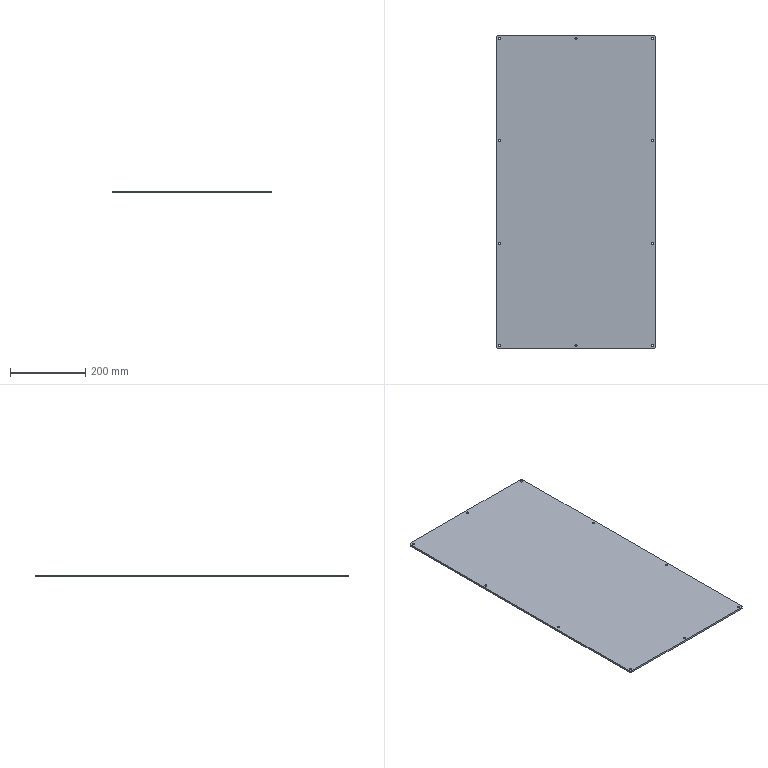Part | NX | features BREP 1 | 1 solid | 30 faces | box 421 x 829 x 5 mm | volume 1743617 mm3 | cylinder 24 | plane 6 | commonest cylinder face diameters 5.8 x20 10 x4
STEP:
#1=CARTESIAN_POINT('',(-205.5,414.5,5.));
#2=VERTEX_POINT('',#1);
#3=CARTESIAN_POINT('',(-210.5,409.5,5.));
#4=VERTEX_POINT('',#3);
#5=CARTESIAN_POINT('',(-205.5,409.5,5.));
#6=DIRECTION('',(0.,0.,1.));
#7=DIRECTION('',(1.,0.,0.));
#8=AXIS2_PLACEMENT_3D('',#5,#6,#7);
#9=CIRCLE('',#8,5.);
#10=EDGE_CURVE('',#2,#4,#9,.T.);
#11=ORIENTED_EDGE('',*,*,#10,.F.);
#12=CARTESIAN_POINT('',(-205.5,414.5,0.));
#13=VERTEX_POINT('',#12);
#14=CARTESIAN_POINT('',(-205.5,414.5,5.));
#15=DIRECTION('',(0.,0.,1.));
#16=VECTOR('',#15,1000.);
#17=LINE('',#14,#16);
#18=EDGE_CURVE('',#13,#2,#17,.T.);
#19=ORIENTED_EDGE('',*,*,#18,.F.);
#20=CARTESIAN_POINT('',(-210.5,409.5,0.));
#21=VERTEX_POINT('',#20);
#22=CARTESIAN_POINT('',(-205.5,409.5,0.));
#23=DIRECTION('',(0.,0.,-1.));
#24=DIRECTION('',(1.,0.,0.));
#25=AXIS2_PLACEMENT_3D('',#22,#23,#24);
#26=CIRCLE('',#25,5.);
#27=EDGE_CURVE('',#21,#13,#26,.T.);
#28=ORIENTED_EDGE('',*,*,#27,.F.);
#29=CARTESIAN_POINT('',(-210.5,409.5,5.));
#30=DIRECTION('',(0.,0.,-1.));
#31=VECTOR('',#30,1000.);
#32=LINE('',#29,#31);
#33=EDGE_CURVE('',#4,#21,#32,.T.);
#34=ORIENTED_EDGE('',*,*,#33,.F.);
#35=EDGE_LOOP('',(#11,#19,#28,#34));
#36=FACE_BOUND('',#35,.T.);
#37=CARTESIAN_POINT('',(-205.5,409.5,5.));
#38=DIRECTION('',(0.,0.,-1.));
#39=DIRECTION('',(-1.,0.,0.));
#40=AXIS2_PLACEMENT_3D('',#37,#38,#39);
#41=CYLINDRICAL_SURFACE('',#40,5.);
#42=ADVANCED_FACE('',(#36),#41,.T.);
#43=CARTESIAN_POINT('',(210.5,409.5,5.));
#44=VERTEX_POINT('',#43);
#45=CARTESIAN_POINT('',(205.5,414.5,5.));
#46=VERTEX_POINT('',#45);
#47=CARTESIAN_POINT('',(205.5,409.5,5.));
#48=DIRECTION('',(0.,0.,1.));
#49=DIRECTION('',(1.,0.,0.));
#50=AXIS2_PLACEMENT_3D('',#47,#48,#49);
#51=CIRCLE('',#50,5.);
#52=EDGE_CURVE('',#44,#46,#51,.T.);
#53=ORIENTED_EDGE('',*,*,#52,.F.);
#54=CARTESIAN_POINT('',(210.5,409.5,0.));
#55=VERTEX_POINT('',#54);
#56=CARTESIAN_POINT('',(210.5,409.5,5.));
#57=DIRECTION('',(0.,0.,1.));
#58=VECTOR('',#57,1000.);
#59=LINE('',#56,#58);
#60=EDGE_CURVE('',#55,#44,#59,.T.);
#61=ORIENTED_EDGE('',*,*,#60,.F.);
#62=CARTESIAN_POINT('',(205.5,414.5,0.));
#63=VERTEX_POINT('',#62);
#64=CARTESIAN_POINT('',(205.5,409.5,0.));
#65=DIRECTION('',(0.,0.,-1.));
#66=DIRECTION('',(1.,0.,0.));
#67=AXIS2_PLACEMENT_3D('',#64,#65,#66);
#68=CIRCLE('',#67,5.);
#69=EDGE_CURVE('',#63,#55,#68,.T.);
#70=ORIENTED_EDGE('',*,*,#69,.F.);
#71=CARTESIAN_POINT('',(205.5,414.5,5.));
#72=DIRECTION('',(0.,0.,-1.));
#73=VECTOR('',#72,1000.);
#74=LINE('',#71,#73);
#75=EDGE_CURVE('',#46,#63,#74,.T.);
#76=ORIENTED_EDGE('',*,*,#75,.F.);
#77=EDGE_LOOP('',(#53,#61,#70,#76));
#78=FACE_BOUND('',#77,.T.);
#79=CARTESIAN_POINT('',(205.5,409.5,5.));
#80=DIRECTION('',(0.,0.,-1.));
#81=DIRECTION('',(-1.,0.,0.));
#82=AXIS2_PLACEMENT_3D('',#79,#80,#81);
#83=CYLINDRICAL_SURFACE('',#82,5.);
#84=ADVANCED_FACE('',(#78),#83,.T.);
#85=CARTESIAN_POINT('',(205.5,-414.5,5.));
#86=VERTEX_POINT('',#85);
#87=CARTESIAN_POINT('',(210.5,-409.5,5.));
#88=VERTEX_POINT('',#87);
#89=CARTESIAN_POINT('',(205.5,-409.5,5.));
#90=DIRECTION('',(0.,0.,1.));
#91=DIRECTION('',(1.,0.,0.));
#92=AXIS2_PLACEMENT_3D('',#89,#90,#91);
#93=CIRCLE('',#92,5.);
#94=EDGE_CURVE('',#86,#88,#93,.T.);
#95=ORIENTED_EDGE('',*,*,#94,.F.);
#96=CARTESIAN_POINT('',(205.5,-414.5,0.));
#97=VERTEX_POINT('',#96);
#98=CARTESIAN_POINT('',(205.5,-414.5,5.));
#99=DIRECTION('',(0.,0.,1.));
#100=VECTOR('',#99,1000.);
#101=LINE('',#98,#100);
#102=EDGE_CURVE('',#97,#86,#101,.T.);
#103=ORIENTED_EDGE('',*,*,#102,.F.);
#104=CARTESIAN_POINT('',(210.5,-409.5,0.));
#105=VERTEX_POINT('',#104);
#106=CARTESIAN_POINT('',(205.5,-409.5,0.));
#107=DIRECTION('',(0.,0.,-1.));
#108=DIRECTION('',(1.,0.,0.));
#109=AXIS2_PLACEMENT_3D('',#106,#107,#108);
#110=CIRCLE('',#109,5.);
#111=EDGE_CURVE('',#105,#97,#110,.T.);
#112=ORIENTED_EDGE('',*,*,#111,.F.);
#113=CARTESIAN_POINT('',(210.5,-409.5,5.));
#114=DIRECTION('',(0.,0.,-1.));
#115=VECTOR('',#114,1000.);
#116=LINE('',#113,#115);
#117=EDGE_CURVE('',#88,#105,#116,.T.);
#118=ORIENTED_EDGE('',*,*,#117,.F.);
#119=EDGE_LOOP('',(#95,#103,#112,#118));
#120=FACE_BOUND('',#119,.T.);
#121=CARTESIAN_POINT('',(205.5,-409.5,5.));
#122=DIRECTION('',(0.,0.,-1.));
#123=DIRECTION('',(-1.,0.,0.));
#124=AXIS2_PLACEMENT_3D('',#121,#122,#123);
#125=CYLINDRICAL_SURFACE('',#124,5.);
#126=ADVANCED_FACE('',(#120),#125,.T.);
#127=CARTESIAN_POINT('',(-210.5,-409.5,5.));
#128=VERTEX_POINT('',#127);
#129=CARTESIAN_POINT('',(-205.5,-414.5,5.));
#130=VERTEX_POINT('',#129);
#131=CARTESIAN_POINT('',(-205.5,-409.5,5.));
#132=DIRECTION('',(0.,0.,1.));
#133=DIRECTION('',(1.,0.,0.));
#134=AXIS2_PLACEMENT_3D('',#131,#132,#133);
#135=CIRCLE('',#134,5.);
#136=EDGE_CURVE('',#128,#130,#135,.T.);
#137=ORIENTED_EDGE('',*,*,#136,.F.);
#138=CARTESIAN_POINT('',(-210.5,-409.5,0.));
#139=VERTEX_POINT('',#138);
#140=CARTESIAN_POINT('',(-210.5,-409.5,5.));
#141=DIRECTION('',(0.,0.,1.));
#142=VECTOR('',#141,1000.);
#143=LINE('',#140,#142);
#144=EDGE_CURVE('',#139,#128,#143,.T.);
#145=ORIENTED_EDGE('',*,*,#144,.F.);
#146=CARTESIAN_POINT('',(-205.5,-414.5,0.));
#147=VERTEX_POINT('',#146);
#148=CARTESIAN_POINT('',(-205.5,-409.5,0.));
#149=DIRECTION('',(0.,0.,-1.));
#150=DIRECTION('',(1.,0.,0.));
#151=AXIS2_PLACEMENT_3D('',#148,#149,#150);
#152=CIRCLE('',#151,5.);
#153=EDGE_CURVE('',#147,#139,#152,.T.);
#154=ORIENTED_EDGE('',*,*,#153,.F.);
#155=CARTESIAN_POINT('',(-205.5,-414.5,5.));
#156=DIRECTION('',(0.,0.,-1.));
#157=VECTOR('',#156,1000.);
#158=LINE('',#155,#157);
#159=EDGE_CURVE('',#130,#147,#158,.T.);
#160=ORIENTED_EDGE('',*,*,#159,.F.);
#161=EDGE_LOOP('',(#137,#145,#154,#160));
#162=FACE_BOUND('',#161,.T.);
#163=CARTESIAN_POINT('',(-205.5,-409.5,5.));
#164=DIRECTION('',(0.,0.,-1.));
#165=DIRECTION('',(-1.,0.,0.));
#166=AXIS2_PLACEMENT_3D('',#163,#164,#165);
#167=CYLINDRICAL_SURFACE('',#166,5.);
#168=ADVANCED_FACE('',(#162),#167,.T.);
#169=CARTESIAN_POINT('',(199.6,-406.5,5.));
#170=VERTEX_POINT('',#169);
#171=CARTESIAN_POINT('',(199.6,-406.5,0.));
#172=VERTEX_POINT('',#171);
#173=CARTESIAN_POINT('',(199.6,-406.5,0.));
#174=DIRECTION('',(0.,0.,1.));
#175=VECTOR('',#174,1000.);
#176=LINE('',#173,#175);
#177=EDGE_CURVE('',#170,#172,#176,.F.);
#178=ORIENTED_EDGE('',*,*,#177,.T.);
#179=CARTESIAN_POINT('',(205.4,-406.5,0.));
#180=VERTEX_POINT('',#179);
#181=CARTESIAN_POINT('',(202.5,-406.5,0.));
#182=DIRECTION('',(0.,0.,1.));
#183=DIRECTION('',(1.,0.,0.));
#184=AXIS2_PLACEMENT_3D('',#181,#182,#183);
#185=CIRCLE('',#184,2.9);
#186=EDGE_CURVE('',#180,#172,#185,.T.);
#187=ORIENTED_EDGE('',*,*,#186,.F.);
#188=CARTESIAN_POINT('',(205.4,-406.5,5.));
#189=VERTEX_POINT('',#188);
#190=CARTESIAN_POINT('',(205.4,-406.5,0.));
#191=DIRECTION('',(0.,0.,1.));
#192=VECTOR('',#191,1000.);
#193=LINE('',#190,#192);
#194=EDGE_CURVE('',#189,#180,#193,.F.);
#195=ORIENTED_EDGE('',*,*,#194,.F.);
#196=CARTESIAN_POINT('',(202.5,-406.5,5.));
#197=DIRECTION('',(0.,0.,1.));
#198=DIRECTION('',(1.,0.,0.));
#199=AXIS2_PLACEMENT_3D('',#196,#197,#198);
#200=CIRCLE('',#199,2.9);
#201=EDGE_CURVE('',#189,#170,#200,.T.);
#202=ORIENTED_EDGE('',*,*,#201,.T.);
#203=EDGE_LOOP('',(#178,#187,#195,#202));
#204=FACE_BOUND('',#203,.T.);
#205=CARTESIAN_POINT('',(202.5,-406.5,0.));
#206=DIRECTION('',(0.,0.,1.));
#207=DIRECTION('',(1.,0.,0.));
#208=AXIS2_PLACEMENT_3D('',#205,#206,#207);
#209=CYLINDRICAL_SURFACE('',#208,2.9);
#210=ADVANCED_FACE('',(#204),#209,.F.);
#211=CARTESIAN_POINT('',(199.6,135.5,5.));
#212=VERTEX_POINT('',#211);
#213=CARTESIAN_POINT('',(199.6,135.5,0.));
#214=VERTEX_POINT('',#213);
#215=CARTESIAN_POINT('',(199.6,135.5,0.));
#216=DIRECTION('',(0.,0.,1.));
#217=VECTOR('',#216,1000.);
#218=LINE('',#215,#217);
#219=EDGE_CURVE('',#212,#214,#218,.F.);
#220=ORIENTED_EDGE('',*,*,#219,.T.);
#221=CARTESIAN_POINT('',(205.4,135.5,0.));
#222=VERTEX_POINT('',#221);
#223=CARTESIAN_POINT('',(202.5,135.5,0.));
#224=DIRECTION('',(0.,0.,1.));
#225=DIRECTION('',(1.,0.,0.));
#226=AXIS2_PLACEMENT_3D('',#223,#224,#225);
#227=CIRCLE('',#226,2.9);
#228=EDGE_CURVE('',#222,#214,#227,.T.);
#229=ORIENTED_EDGE('',*,*,#228,.F.);
#230=CARTESIAN_POINT('',(205.4,135.5,5.));
#231=VERTEX_POINT('',#230);
#232=CARTESIAN_POINT('',(205.4,135.5,0.));
#233=DIRECTION('',(0.,0.,1.));
#234=VECTOR('',#233,1000.);
#235=LINE('',#232,#234);
#236=EDGE_CURVE('',#231,#222,#235,.F.);
#237=ORIENTED_EDGE('',*,*,#236,.F.);
#238=CARTESIAN_POINT('',(202.5,135.5,5.));
#239=DIRECTION('',(0.,0.,1.));
#240=DIRECTION('',(1.,0.,0.));
#241=AXIS2_PLACEMENT_3D('',#238,#239,#240);
#242=CIRCLE('',#241,2.9);
#243=EDGE_CURVE('',#231,#212,#242,.T.);
#244=ORIENTED_EDGE('',*,*,#243,.T.);
#245=EDGE_LOOP('',(#220,#229,#237,#244));
#246=FACE_BOUND('',#245,.T.);
#247=CARTESIAN_POINT('',(202.5,135.5,0.));
#248=DIRECTION('',(0.,0.,1.));
#249=DIRECTION('',(1.,0.,0.));
#250=AXIS2_PLACEMENT_3D('',#247,#248,#249);
#251=CYLINDRICAL_SURFACE('',#250,2.9);
#252=ADVANCED_FACE('',(#246),#251,.F.);
#253=CARTESIAN_POINT('',(199.6,-135.5,5.));
#254=VERTEX_POINT('',#253);
#255=CARTESIAN_POINT('',(199.6,-135.5,0.));
#256=VERTEX_POINT('',#255);
#257=CARTESIAN_POINT('',(199.6,-135.5,0.));
#258=DIRECTION('',(0.,0.,1.));
#259=VECTOR('',#258,1000.);
#260=LINE('',#257,#259);
#261=EDGE_CURVE('',#254,#256,#260,.F.);
#262=ORIENTED_EDGE('',*,*,#261,.T.);
#263=CARTESIAN_POINT('',(205.4,-135.5,0.));
#264=VERTEX_POINT('',#263);
#265=CARTESIAN_POINT('',(202.5,-135.5,0.));
#266=DIRECTION('',(0.,0.,1.));
#267=DIRECTION('',(1.,0.,0.));
#268=AXIS2_PLACEMENT_3D('',#265,#266,#267);
#269=CIRCLE('',#268,2.9);
#270=EDGE_CURVE('',#264,#256,#269,.T.);
#271=ORIENTED_EDGE('',*,*,#270,.F.);
#272=CARTESIAN_POINT('',(205.4,-135.5,5.));
#273=VERTEX_POINT('',#272);
#274=CARTESIAN_POINT('',(205.4,-135.5,0.));
#275=DIRECTION('',(0.,0.,1.));
#276=VECTOR('',#275,1000.);
#277=LINE('',#274,#276);
#278=EDGE_CURVE('',#273,#264,#277,.F.);
#279=ORIENTED_EDGE('',*,*,#278,.F.);
#280=CARTESIAN_POINT('',(202.5,-135.5,5.));
#281=DIRECTION('',(0.,0.,1.));
#282=DIRECTION('',(1.,0.,0.));
#283=AXIS2_PLACEMENT_3D('',#280,#281,#282);
#284=CIRCLE('',#283,2.9);
#285=EDGE_CURVE('',#273,#254,#284,.T.);
#286=ORIENTED_EDGE('',*,*,#285,.T.);
#287=EDGE_LOOP('',(#262,#271,#279,#286));
#288=FACE_BOUND('',#287,.T.);
#289=CARTESIAN_POINT('',(202.5,-135.5,0.));
#290=DIRECTION('',(0.,0.,1.));
#291=DIRECTION('',(1.,0.,0.));
#292=AXIS2_PLACEMENT_3D('',#289,#290,#291);
#293=CYLINDRICAL_SURFACE('',#292,2.9);
#294=ADVANCED_FACE('',(#288),#293,.F.);
#295=CARTESIAN_POINT('',(-205.4,135.5,5.));
#296=VERTEX_POINT('',#295);
#297=CARTESIAN_POINT('',(-205.4,135.5,0.));
#298=VERTEX_POINT('',#297);
#299=CARTESIAN_POINT('',(-205.4,135.5,0.));
#300=DIRECTION('',(0.,0.,1.));
#301=VECTOR('',#300,1000.);
#302=LINE('',#299,#301);
#303=EDGE_CURVE('',#296,#298,#302,.F.);
#304=ORIENTED_EDGE('',*,*,#303,.T.);
#305=CARTESIAN_POINT('',(-199.6,135.5,0.));
#306=VERTEX_POINT('',#305);
#307=CARTESIAN_POINT('',(-202.5,135.5,0.));
#308=DIRECTION('',(0.,0.,1.));
#309=DIRECTION('',(1.,0.,0.));
#310=AXIS2_PLACEMENT_3D('',#307,#308,#309);
#311=CIRCLE('',#310,2.9);
#312=EDGE_CURVE('',#306,#298,#311,.T.);
#313=ORIENTED_EDGE('',*,*,#312,.F.);
#314=CARTESIAN_POINT('',(-199.6,135.5,5.));
#315=VERTEX_POINT('',#314);
#316=CARTESIAN_POINT('',(-199.6,135.5,0.));
#317=DIRECTION('',(0.,0.,1.));
#318=VECTOR('',#317,1000.);
#319=LINE('',#316,#318);
#320=EDGE_CURVE('',#315,#306,#319,.F.);
#321=ORIENTED_EDGE('',*,*,#320,.F.);
#322=CARTESIAN_POINT('',(-202.5,135.5,5.));
#323=DIRECTION('',(0.,0.,1.));
#324=DIRECTION('',(1.,0.,0.));
#325=AXIS2_PLACEMENT_3D('',#322,#323,#324);
#326=CIRCLE('',#325,2.9);
#327=EDGE_CURVE('',#315,#296,#326,.T.);
#328=ORIENTED_EDGE('',*,*,#327,.T.);
#329=EDGE_LOOP('',(#304,#313,#321,#328));
#330=FACE_BOUND('',#329,.T.);
#331=CARTESIAN_POINT('',(-202.5,135.5,0.));
#332=DIRECTION('',(0.,0.,1.));
#333=DIRECTION('',(1.,0.,0.));
#334=AXIS2_PLACEMENT_3D('',#331,#332,#333);
#335=CYLINDRICAL_SURFACE('',#334,2.9);
#336=ADVANCED_FACE('',(#330),#335,.F.);
#337=CARTESIAN_POINT('',(-2.9,-406.5,5.));
#338=VERTEX_POINT('',#337);
#339=CARTESIAN_POINT('',(-2.9,-406.5,0.));
#340=VERTEX_POINT('',#339);
#341=CARTESIAN_POINT('',(-2.9,-406.5,0.));
#342=DIRECTION('',(0.,0.,1.));
#343=VECTOR('',#342,1000.);
#344=LINE('',#341,#343);
#345=EDGE_CURVE('',#338,#340,#344,.F.);
#346=ORIENTED_EDGE('',*,*,#345,.T.);
#347=CARTESIAN_POINT('',(2.9,-406.5,0.));
#348=VERTEX_POINT('',#347);
#349=CARTESIAN_POINT('',(0.,-406.5,0.));
#350=DIRECTION('',(0.,0.,1.));
#351=DIRECTION('',(1.,0.,0.));
#352=AXIS2_PLACEMENT_3D('',#349,#350,#351);
#353=CIRCLE('',#352,2.9);
#354=EDGE_CURVE('',#348,#340,#353,.T.);
#355=ORIENTED_EDGE('',*,*,#354,.F.);
#356=CARTESIAN_POINT('',(2.9,-406.5,5.));
#357=VERTEX_POINT('',#356);
#358=CARTESIAN_POINT('',(2.9,-406.5,0.));
#359=DIRECTION('',(0.,0.,1.));
#360=VECTOR('',#359,1000.);
#361=LINE('',#358,#360);
#362=EDGE_CURVE('',#357,#348,#361,.F.);
#363=ORIENTED_EDGE('',*,*,#362,.F.);
#364=CARTESIAN_POINT('',(0.,-406.5,5.));
#365=DIRECTION('',(0.,0.,1.));
#366=DIRECTION('',(1.,0.,0.));
#367=AXIS2_PLACEMENT_3D('',#364,#365,#366);
#368=CIRCLE('',#367,2.9);
#369=EDGE_CURVE('',#357,#338,#368,.T.);
#370=ORIENTED_EDGE('',*,*,#369,.T.);
#371=EDGE_LOOP('',(#346,#355,#363,#370));
#372=FACE_BOUND('',#371,.T.);
#373=CARTESIAN_POINT('',(0.,-406.5,0.));
#374=DIRECTION('',(0.,0.,1.));
#375=DIRECTION('',(1.,0.,0.));
#376=AXIS2_PLACEMENT_3D('',#373,#374,#375);
#377=CYLINDRICAL_SURFACE('',#376,2.9);
#378=ADVANCED_FACE('',(#372),#377,.F.);
#379=CARTESIAN_POINT('',(-205.4,-406.5,5.));
#380=VERTEX_POINT('',#379);
#381=CARTESIAN_POINT('',(-205.4,-406.5,0.));
#382=VERTEX_POINT('',#381);
#383=CARTESIAN_POINT('',(-205.4,-406.5,0.));
#384=DIRECTION('',(0.,0.,1.));
#385=VECTOR('',#384,1000.);
#386=LINE('',#383,#385);
#387=EDGE_CURVE('',#380,#382,#386,.F.);
#388=ORIENTED_EDGE('',*,*,#387,.T.);
#389=CARTESIAN_POINT('',(-199.6,-406.5,0.));
#390=VERTEX_POINT('',#389);
#391=CARTESIAN_POINT('',(-202.5,-406.5,0.));
#392=DIRECTION('',(0.,0.,1.));
#393=DIRECTION('',(1.,0.,0.));
#394=AXIS2_PLACEMENT_3D('',#391,#392,#393);
#395=CIRCLE('',#394,2.9);
#396=EDGE_CURVE('',#390,#382,#395,.T.);
#397=ORIENTED_EDGE('',*,*,#396,.F.);
#398=CARTESIAN_POINT('',(-199.6,-406.5,5.));
#399=VERTEX_POINT('',#398);
#400=CARTESIAN_POINT('',(-199.6,-406.5,0.));
#401=DIRECTION('',(0.,0.,1.));
#402=VECTOR('',#401,1000.);
#403=LINE('',#400,#402);
#404=EDGE_CURVE('',#399,#390,#403,.F.);
#405=ORIENTED_EDGE('',*,*,#404,.F.);
#406=CARTESIAN_POINT('',(-202.5,-406.5,5.));
#407=DIRECTION('',(0.,0.,1.));
#408=DIRECTION('',(1.,0.,0.));
#409=AXIS2_PLACEMENT_3D('',#406,#407,#408);
#410=CIRCLE('',#409,2.9);
#411=EDGE_CURVE('',#399,#380,#410,.T.);
#412=ORIENTED_EDGE('',*,*,#411,.T.);
#413=EDGE_LOOP('',(#388,#397,#405,#412));
#414=FACE_BOUND('',#413,.T.);
#415=CARTESIAN_POINT('',(-202.5,-406.5,0.));
#416=DIRECTION('',(0.,0.,1.));
#417=DIRECTION('',(1.,0.,0.));
#418=AXIS2_PLACEMENT_3D('',#415,#416,#417);
#419=CYLINDRICAL_SURFACE('',#418,2.9);
#420=ADVANCED_FACE('',(#414),#419,.F.);
#421=CARTESIAN_POINT('',(199.6,406.5,5.));
#422=VERTEX_POINT('',#421);
#423=CARTESIAN_POINT('',(199.6,406.5,0.));
#424=VERTEX_POINT('',#423);
#425=CARTESIAN_POINT('',(199.6,406.5,0.));
#426=DIRECTION('',(0.,0.,1.));
#427=VECTOR('',#426,1000.);
#428=LINE('',#425,#427);
#429=EDGE_CURVE('',#422,#424,#428,.F.);
#430=ORIENTED_EDGE('',*,*,#429,.T.);
#431=CARTESIAN_POINT('',(205.4,406.5,0.));
#432=VERTEX_POINT('',#431);
#433=CARTESIAN_POINT('',(202.5,406.5,0.));
#434=DIRECTION('',(0.,0.,1.));
#435=DIRECTION('',(1.,0.,0.));
#436=AXIS2_PLACEMENT_3D('',#433,#434,#435);
#437=CIRCLE('',#436,2.9);
#438=EDGE_CURVE('',#432,#424,#437,.T.);
#439=ORIENTED_EDGE('',*,*,#438,.F.);
#440=CARTESIAN_POINT('',(205.4,406.5,5.));
#441=VERTEX_POINT('',#440);
#442=CARTESIAN_POINT('',(205.4,406.5,0.));
#443=DIRECTION('',(0.,0.,1.));
#444=VECTOR('',#443,1000.);
#445=LINE('',#442,#444);
#446=EDGE_CURVE('',#441,#432,#445,.F.);
#447=ORIENTED_EDGE('',*,*,#446,.F.);
#448=CARTESIAN_POINT('',(202.5,406.5,5.));
#449=DIRECTION('',(0.,0.,1.));
#450=DIRECTION('',(1.,0.,0.));
#451=AXIS2_PLACEMENT_3D('',#448,#449,#450);
#452=CIRCLE('',#451,2.9);
#453=EDGE_CURVE('',#441,#422,#452,.T.);
#454=ORIENTED_EDGE('',*,*,#453,.T.);
#455=EDGE_LOOP('',(#430,#439,#447,#454));
#456=FACE_BOUND('',#455,.T.);
#457=CARTESIAN_POINT('',(202.5,406.5,0.));
#458=DIRECTION('',(0.,0.,1.));
#459=DIRECTION('',(1.,0.,0.));
#460=AXIS2_PLACEMENT_3D('',#457,#458,#459);
#461=CYLINDRICAL_SURFACE('',#460,2.9);
#462=ADVANCED_FACE('',(#456),#461,.F.);
#463=CARTESIAN_POINT('',(-2.9,406.5,5.));
#464=VERTEX_POINT('',#463);
#465=CARTESIAN_POINT('',(-2.9,406.5,0.));
#466=VERTEX_POINT('',#465);
#467=CARTESIAN_POINT('',(-2.9,406.5,0.));
#468=DIRECTION('',(0.,0.,1.));
#469=VECTOR('',#468,1000.);
#470=LINE('',#467,#469);
#471=EDGE_CURVE('',#464,#466,#470,.F.);
#472=ORIENTED_EDGE('',*,*,#471,.T.);
#473=CARTESIAN_POINT('',(2.9,406.5,0.));
#474=VERTEX_POINT('',#473);
#475=CARTESIAN_POINT('',(0.,406.5,0.));
#476=DIRECTION('',(0.,0.,1.));
#477=DIRECTION('',(1.,0.,0.));
#478=AXIS2_PLACEMENT_3D('',#475,#476,#477);
#479=CIRCLE('',#478,2.9);
#480=EDGE_CURVE('',#474,#466,#479,.T.);
#481=ORIENTED_EDGE('',*,*,#480,.F.);
#482=CARTESIAN_POINT('',(2.9,406.5,5.));
#483=VERTEX_POINT('',#482);
#484=CARTESIAN_POINT('',(2.9,406.5,0.));
#485=DIRECTION('',(0.,0.,1.));
#486=VECTOR('',#485,1000.);
#487=LINE('',#484,#486);
#488=EDGE_CURVE('',#483,#474,#487,.F.);
#489=ORIENTED_EDGE('',*,*,#488,.F.);
#490=CARTESIAN_POINT('',(0.,406.5,5.));
#491=DIRECTION('',(0.,0.,1.));
#492=DIRECTION('',(1.,0.,0.));
#493=AXIS2_PLACEMENT_3D('',#490,#491,#492);
#494=CIRCLE('',#493,2.9);
#495=EDGE_CURVE('',#483,#464,#494,.T.);
#496=ORIENTED_EDGE('',*,*,#495,.T.);
#497=EDGE_LOOP('',(#472,#481,#489,#496));
#498=FACE_BOUND('',#497,.T.);
#499=CARTESIAN_POINT('',(0.,406.5,0.));
#500=DIRECTION('',(0.,0.,1.));
#501=DIRECTION('',(1.,0.,0.));
#502=AXIS2_PLACEMENT_3D('',#499,#500,#501);
#503=CYLINDRICAL_SURFACE('',#502,2.9);
#504=ADVANCED_FACE('',(#498),#503,.F.);
#505=CARTESIAN_POINT('',(-205.4,-135.5,5.));
#506=VERTEX_POINT('',#505);
#507=CARTESIAN_POINT('',(-205.4,-135.5,0.));
#508=VERTEX_POINT('',#507);
#509=CARTESIAN_POINT('',(-205.4,-135.5,0.));
#510=DIRECTION('',(0.,0.,1.));
#511=VECTOR('',#510,1000.);
#512=LINE('',#509,#511);
#513=EDGE_CURVE('',#506,#508,#512,.F.);
#514=ORIENTED_EDGE('',*,*,#513,.T.);
#515=CARTESIAN_POINT('',(-199.6,-135.5,0.));
#516=VERTEX_POINT('',#515);
#517=CARTESIAN_POINT('',(-202.5,-135.5,0.));
#518=DIRECTION('',(0.,0.,1.));
#519=DIRECTION('',(1.,0.,0.));
#520=AXIS2_PLACEMENT_3D('',#517,#518,#519);
#521=CIRCLE('',#520,2.9);
#522=EDGE_CURVE('',#516,#508,#521,.T.);
#523=ORIENTED_EDGE('',*,*,#522,.F.);
#524=CARTESIAN_POINT('',(-199.6,-135.5,5.));
#525=VERTEX_POINT('',#524);
#526=CARTESIAN_POINT('',(-199.6,-135.5,0.));
#527=DIRECTION('',(0.,0.,1.));
#528=VECTOR('',#527,1000.);
#529=LINE('',#526,#528);
#530=EDGE_CURVE('',#525,#516,#529,.F.);
#531=ORIENTED_EDGE('',*,*,#530,.F.);
#532=CARTESIAN_POINT('',(-202.5,-135.5,5.));
#533=DIRECTION('',(0.,0.,1.));
#534=DIRECTION('',(1.,0.,0.));
#535=AXIS2_PLACEMENT_3D('',#532,#533,#534);
#536=CIRCLE('',#535,2.9);
#537=EDGE_CURVE('',#525,#506,#536,.T.);
#538=ORIENTED_EDGE('',*,*,#537,.T.);
#539=EDGE_LOOP('',(#514,#523,#531,#538));
#540=FACE_BOUND('',#539,.T.);
#541=CARTESIAN_POINT('',(-202.5,-135.5,0.));
#542=DIRECTION('',(0.,0.,1.));
#543=DIRECTION('',(1.,0.,0.));
#544=AXIS2_PLACEMENT_3D('',#541,#542,#543);
#545=CYLINDRICAL_SURFACE('',#544,2.9);
#546=ADVANCED_FACE('',(#540),#545,.F.);
#547=CARTESIAN_POINT('',(-205.4,406.5,5.));
#548=VERTEX_POINT('',#547);
#549=CARTESIAN_POINT('',(-205.4,406.5,0.));
#550=VERTEX_POINT('',#549);
#551=CARTESIAN_POINT('',(-205.4,406.5,0.));
#552=DIRECTION('',(0.,0.,1.));
#553=VECTOR('',#552,1000.);
#554=LINE('',#551,#553);
#555=EDGE_CURVE('',#548,#550,#554,.F.);
#556=ORIENTED_EDGE('',*,*,#555,.T.);
#557=CARTESIAN_POINT('',(-199.6,406.5,0.));
#558=VERTEX_POINT('',#557);
#559=CARTESIAN_POINT('',(-202.5,406.5,0.));
#560=DIRECTION('',(0.,0.,1.));
#561=DIRECTION('',(1.,0.,0.));
#562=AXIS2_PLACEMENT_3D('',#559,#560,#561);
#563=CIRCLE('',#562,2.9);
#564=EDGE_CURVE('',#558,#550,#563,.T.);
#565=ORIENTED_EDGE('',*,*,#564,.F.);
#566=CARTESIAN_POINT('',(-199.6,406.5,5.));
#567=VERTEX_POINT('',#566);
#568=CARTESIAN_POINT('',(-199.6,406.5,0.));
#569=DIRECTION('',(0.,0.,1.));
#570=VECTOR('',#569,1000.);
#571=LINE('',#568,#570);
#572=EDGE_CURVE('',#567,#558,#571,.F.);
#573=ORIENTED_EDGE('',*,*,#572,.F.);
#574=CARTESIAN_POINT('',(-202.5,406.5,5.));
#575=DIRECTION('',(0.,0.,1.));
#576=DIRECTION('',(1.,0.,0.));
#577=AXIS2_PLACEMENT_3D('',#574,#575,#576);
#578=CIRCLE('',#577,2.9);
#579=EDGE_CURVE('',#567,#548,#578,.T.);
#580=ORIENTED_EDGE('',*,*,#579,.T.);
#581=EDGE_LOOP('',(#556,#565,#573,#580));
#582=FACE_BOUND('',#581,.T.);
#583=CARTESIAN_POINT('',(-202.5,406.5,0.));
#584=DIRECTION('',(0.,0.,1.));
#585=DIRECTION('',(1.,0.,0.));
#586=AXIS2_PLACEMENT_3D('',#583,#584,#585);
#587=CYLINDRICAL_SURFACE('',#586,2.9);
#588=ADVANCED_FACE('',(#582),#587,.F.);
#589=CARTESIAN_POINT('',(210.5,-414.5,0.));
#590=DIRECTION('',(1.,0.,0.));
#591=VECTOR('',#590,1000.);
#592=LINE('',#589,#591);
#593=EDGE_CURVE('',#147,#97,#592,.T.);
#594=ORIENTED_EDGE('',*,*,#593,.F.);
#595=ORIENTED_EDGE('',*,*,#153,.T.);
#596=CARTESIAN_POINT('',(-210.5,-414.5,0.));
#597=DIRECTION('',(0.,-1.,0.));
#598=VECTOR('',#597,1000.);
#599=LINE('',#596,#598);
#600=EDGE_CURVE('',#21,#139,#599,.T.);
#601=ORIENTED_EDGE('',*,*,#600,.F.);
#602=ORIENTED_EDGE('',*,*,#27,.T.);
#603=CARTESIAN_POINT('',(210.5,414.5,0.));
#604=DIRECTION('',(-1.,0.,0.));
#605=VECTOR('',#604,1000.);
#606=LINE('',#603,#605);
#607=EDGE_CURVE('',#63,#13,#606,.T.);
#608=ORIENTED_EDGE('',*,*,#607,.F.);
#609=ORIENTED_EDGE('',*,*,#69,.T.);
#610=CARTESIAN_POINT('',(210.5,-414.5,0.));
#611=DIRECTION('',(0.,1.,0.));
#612=VECTOR('',#611,1000.);
#613=LINE('',#610,#612);
#614=EDGE_CURVE('',#105,#55,#613,.T.);
#615=ORIENTED_EDGE('',*,*,#614,.F.);
#616=ORIENTED_EDGE('',*,*,#111,.T.);
#617=EDGE_LOOP('',(#594,#595,#601,#602,#608,#609,#615,#616));
#618=FACE_BOUND('',#617,.T.);
#619=ORIENTED_EDGE('',*,*,#564,.T.);
#620=CARTESIAN_POINT('',(-202.5,406.5,0.));
#621=DIRECTION('',(0.,0.,1.));
#622=DIRECTION('',(1.,0.,0.));
#623=AXIS2_PLACEMENT_3D('',#620,#621,#622);
#624=CIRCLE('',#623,2.9);
#625=EDGE_CURVE('',#550,#558,#624,.T.);
#626=ORIENTED_EDGE('',*,*,#625,.T.);
#627=EDGE_LOOP('',(#619,#626));
#628=FACE_BOUND('',#627,.T.);
#629=ORIENTED_EDGE('',*,*,#522,.T.);
#630=CARTESIAN_POINT('',(-202.5,-135.5,0.));
#631=DIRECTION('',(0.,0.,1.));
#632=DIRECTION('',(1.,0.,0.));
#633=AXIS2_PLACEMENT_3D('',#630,#631,#632);
#634=CIRCLE('',#633,2.9);
#635=EDGE_CURVE('',#508,#516,#634,.T.);
#636=ORIENTED_EDGE('',*,*,#635,.T.);
#637=EDGE_LOOP('',(#629,#636));
#638=FACE_BOUND('',#637,.T.);
#639=ORIENTED_EDGE('',*,*,#480,.T.);
#640=CARTESIAN_POINT('',(0.,406.5,0.));
#641=DIRECTION('',(0.,0.,1.));
#642=DIRECTION('',(1.,0.,0.));
#643=AXIS2_PLACEMENT_3D('',#640,#641,#642);
#644=CIRCLE('',#643,2.9);
#645=EDGE_CURVE('',#466,#474,#644,.T.);
#646=ORIENTED_EDGE('',*,*,#645,.T.);
#647=EDGE_LOOP('',(#639,#646));
#648=FACE_BOUND('',#647,.T.);
#649=ORIENTED_EDGE('',*,*,#438,.T.);
#650=CARTESIAN_POINT('',(202.5,406.5,0.));
#651=DIRECTION('',(0.,0.,1.));
#652=DIRECTION('',(1.,0.,0.));
#653=AXIS2_PLACEMENT_3D('',#650,#651,#652);
#654=CIRCLE('',#653,2.9);
#655=EDGE_CURVE('',#424,#432,#654,.T.);
#656=ORIENTED_EDGE('',*,*,#655,.T.);
#657=EDGE_LOOP('',(#649,#656));
#658=FACE_BOUND('',#657,.T.);
#659=ORIENTED_EDGE('',*,*,#396,.T.);
#660=CARTESIAN_POINT('',(-202.5,-406.5,0.));
#661=DIRECTION('',(0.,0.,1.));
#662=DIRECTION('',(1.,0.,0.));
#663=AXIS2_PLACEMENT_3D('',#660,#661,#662);
#664=CIRCLE('',#663,2.9);
#665=EDGE_CURVE('',#382,#390,#664,.T.);
#666=ORIENTED_EDGE('',*,*,#665,.T.);
#667=EDGE_LOOP('',(#659,#666));
#668=FACE_BOUND('',#667,.T.);
#669=ORIENTED_EDGE('',*,*,#354,.T.);
#670=CARTESIAN_POINT('',(0.,-406.5,0.));
#671=DIRECTION('',(0.,0.,1.));
#672=DIRECTION('',(1.,0.,0.));
#673=AXIS2_PLACEMENT_3D('',#670,#671,#672);
#674=CIRCLE('',#673,2.9);
#675=EDGE_CURVE('',#340,#348,#674,.T.);
#676=ORIENTED_EDGE('',*,*,#675,.T.);
#677=EDGE_LOOP('',(#669,#676));
#678=FACE_BOUND('',#677,.T.);
#679=ORIENTED_EDGE('',*,*,#312,.T.);
#680=CARTESIAN_POINT('',(-202.5,135.5,0.));
#681=DIRECTION('',(0.,0.,1.));
#682=DIRECTION('',(1.,0.,0.));
#683=AXIS2_PLACEMENT_3D('',#680,#681,#682);
#684=CIRCLE('',#683,2.9);
#685=EDGE_CURVE('',#298,#306,#684,.T.);
#686=ORIENTED_EDGE('',*,*,#685,.T.);
#687=EDGE_LOOP('',(#679,#686));
#688=FACE_BOUND('',#687,.T.);
#689=ORIENTED_EDGE('',*,*,#270,.T.);
#690=CARTESIAN_POINT('',(202.5,-135.5,0.));
#691=DIRECTION('',(0.,0.,1.));
#692=DIRECTION('',(1.,0.,0.));
#693=AXIS2_PLACEMENT_3D('',#690,#691,#692);
#694=CIRCLE('',#693,2.9);
#695=EDGE_CURVE('',#256,#264,#694,.T.);
#696=ORIENTED_EDGE('',*,*,#695,.T.);
#697=EDGE_LOOP('',(#689,#696));
#698=FACE_BOUND('',#697,.T.);
#699=ORIENTED_EDGE('',*,*,#228,.T.);
#700=CARTESIAN_POINT('',(202.5,135.5,0.));
#701=DIRECTION('',(0.,0.,1.));
#702=DIRECTION('',(1.,0.,0.));
#703=AXIS2_PLACEMENT_3D('',#700,#701,#702);
#704=CIRCLE('',#703,2.9);
#705=EDGE_CURVE('',#214,#222,#704,.T.);
#706=ORIENTED_EDGE('',*,*,#705,.T.);
#707=EDGE_LOOP('',(#699,#706));
#708=FACE_BOUND('',#707,.T.);
#709=ORIENTED_EDGE('',*,*,#186,.T.);
#710=CARTESIAN_POINT('',(202.5,-406.5,0.));
#711=DIRECTION('',(0.,0.,1.));
#712=DIRECTION('',(1.,0.,0.));
#713=AXIS2_PLACEMENT_3D('',#710,#711,#712);
#714=CIRCLE('',#713,2.9);
#715=EDGE_CURVE('',#172,#180,#714,.T.);
#716=ORIENTED_EDGE('',*,*,#715,.T.);
#717=EDGE_LOOP('',(#709,#716));
#718=FACE_BOUND('',#717,.T.);
#719=CARTESIAN_POINT('',(0.,0.,0.));
#720=DIRECTION('',(0.,0.,1.));
#721=DIRECTION('',(1.,0.,0.));
#722=AXIS2_PLACEMENT_3D('',#719,#720,#721);
#723=PLANE('',#722);
#724=ADVANCED_FACE('',(#618,#628,#638,#648,#658,#668,#678,#688,#698,#708,#718),#723,.F.);
#725=CARTESIAN_POINT('',(-210.5,-414.5,5.));
#726=DIRECTION('',(0.,-1.,0.));
#727=VECTOR('',#726,1000.);
#728=LINE('',#725,#727);
#729=EDGE_CURVE('',#4,#128,#728,.T.);
#730=ORIENTED_EDGE('',*,*,#729,.T.);
#731=ORIENTED_EDGE('',*,*,#136,.T.);
#732=CARTESIAN_POINT('',(210.5,-414.5,5.));
#733=DIRECTION('',(1.,0.,0.));
#734=VECTOR('',#733,1000.);
#735=LINE('',#732,#734);
#736=EDGE_CURVE('',#130,#86,#735,.T.);
#737=ORIENTED_EDGE('',*,*,#736,.T.);
#738=ORIENTED_EDGE('',*,*,#94,.T.);
#739=CARTESIAN_POINT('',(210.5,-414.5,5.));
#740=DIRECTION('',(0.,1.,0.));
#741=VECTOR('',#740,1000.);
#742=LINE('',#739,#741);
#743=EDGE_CURVE('',#88,#44,#742,.T.);
#744=ORIENTED_EDGE('',*,*,#743,.T.);
#745=ORIENTED_EDGE('',*,*,#52,.T.);
#746=CARTESIAN_POINT('',(210.5,414.5,5.));
#747=DIRECTION('',(-1.,0.,0.));
#748=VECTOR('',#747,1000.);
#749=LINE('',#746,#748);
#750=EDGE_CURVE('',#46,#2,#749,.T.);
#751=ORIENTED_EDGE('',*,*,#750,.T.);
#752=ORIENTED_EDGE('',*,*,#10,.T.);
#753=EDGE_LOOP('',(#730,#731,#737,#738,#744,#745,#751,#752));
#754=FACE_BOUND('',#753,.T.);
#755=ORIENTED_EDGE('',*,*,#579,.F.);
#756=CARTESIAN_POINT('',(-202.5,406.5,5.));
#757=DIRECTION('',(0.,0.,1.));
#758=DIRECTION('',(1.,0.,0.));
#759=AXIS2_PLACEMENT_3D('',#756,#757,#758);
#760=CIRCLE('',#759,2.9);
#761=EDGE_CURVE('',#548,#567,#760,.T.);
#762=ORIENTED_EDGE('',*,*,#761,.F.);
#763=EDGE_LOOP('',(#755,#762));
#764=FACE_BOUND('',#763,.T.);
#765=ORIENTED_EDGE('',*,*,#537,.F.);
#766=CARTESIAN_POINT('',(-202.5,-135.5,5.));
#767=DIRECTION('',(0.,0.,1.));
#768=DIRECTION('',(1.,0.,0.));
#769=AXIS2_PLACEMENT_3D('',#766,#767,#768);
#770=CIRCLE('',#769,2.9);
#771=EDGE_CURVE('',#506,#525,#770,.T.);
#772=ORIENTED_EDGE('',*,*,#771,.F.);
#773=EDGE_LOOP('',(#765,#772));
#774=FACE_BOUND('',#773,.T.);
#775=ORIENTED_EDGE('',*,*,#495,.F.);
#776=CARTESIAN_POINT('',(0.,406.5,5.));
#777=DIRECTION('',(0.,0.,1.));
#778=DIRECTION('',(1.,0.,0.));
#779=AXIS2_PLACEMENT_3D('',#776,#777,#778);
#780=CIRCLE('',#779,2.9);
#781=EDGE_CURVE('',#464,#483,#780,.T.);
#782=ORIENTED_EDGE('',*,*,#781,.F.);
#783=EDGE_LOOP('',(#775,#782));
#784=FACE_BOUND('',#783,.T.);
#785=ORIENTED_EDGE('',*,*,#453,.F.);
#786=CARTESIAN_POINT('',(202.5,406.5,5.));
#787=DIRECTION('',(0.,0.,1.));
#788=DIRECTION('',(1.,0.,0.));
#789=AXIS2_PLACEMENT_3D('',#786,#787,#788);
#790=CIRCLE('',#789,2.9);
#791=EDGE_CURVE('',#422,#441,#790,.T.);
#792=ORIENTED_EDGE('',*,*,#791,.F.);
#793=EDGE_LOOP('',(#785,#792));
#794=FACE_BOUND('',#793,.T.);
#795=ORIENTED_EDGE('',*,*,#411,.F.);
#796=CARTESIAN_POINT('',(-202.5,-406.5,5.));
#797=DIRECTION('',(0.,0.,1.));
#798=DIRECTION('',(1.,0.,0.));
#799=AXIS2_PLACEMENT_3D('',#796,#797,#798);
#800=CIRCLE('',#799,2.9);
#801=EDGE_CURVE('',#380,#399,#800,.T.);
#802=ORIENTED_EDGE('',*,*,#801,.F.);
#803=EDGE_LOOP('',(#795,#802));
#804=FACE_BOUND('',#803,.T.);
#805=ORIENTED_EDGE('',*,*,#369,.F.);
#806=CARTESIAN_POINT('',(0.,-406.5,5.));
#807=DIRECTION('',(0.,0.,1.));
#808=DIRECTION('',(1.,0.,0.));
#809=AXIS2_PLACEMENT_3D('',#806,#807,#808);
#810=CIRCLE('',#809,2.9);
#811=EDGE_CURVE('',#338,#357,#810,.T.);
#812=ORIENTED_EDGE('',*,*,#811,.F.);
#813=EDGE_LOOP('',(#805,#812));
#814=FACE_BOUND('',#813,.T.);
#815=ORIENTED_EDGE('',*,*,#327,.F.);
#816=CARTESIAN_POINT('',(-202.5,135.5,5.));
#817=DIRECTION('',(0.,0.,1.));
#818=DIRECTION('',(1.,0.,0.));
#819=AXIS2_PLACEMENT_3D('',#816,#817,#818);
#820=CIRCLE('',#819,2.9);
#821=EDGE_CURVE('',#296,#315,#820,.T.);
#822=ORIENTED_EDGE('',*,*,#821,.F.);
#823=EDGE_LOOP('',(#815,#822));
#824=FACE_BOUND('',#823,.T.);
#825=ORIENTED_EDGE('',*,*,#285,.F.);
#826=CARTESIAN_POINT('',(202.5,-135.5,5.));
#827=DIRECTION('',(0.,0.,1.));
#828=DIRECTION('',(1.,0.,0.));
#829=AXIS2_PLACEMENT_3D('',#826,#827,#828);
#830=CIRCLE('',#829,2.9);
#831=EDGE_CURVE('',#254,#273,#830,.T.);
#832=ORIENTED_EDGE('',*,*,#831,.F.);
#833=EDGE_LOOP('',(#825,#832));
#834=FACE_BOUND('',#833,.T.);
#835=ORIENTED_EDGE('',*,*,#243,.F.);
#836=CARTESIAN_POINT('',(202.5,135.5,5.));
#837=DIRECTION('',(0.,0.,1.));
#838=DIRECTION('',(1.,0.,0.));
#839=AXIS2_PLACEMENT_3D('',#836,#837,#838);
#840=CIRCLE('',#839,2.9);
#841=EDGE_CURVE('',#212,#231,#840,.T.);
#842=ORIENTED_EDGE('',*,*,#841,.F.);
#843=EDGE_LOOP('',(#835,#842));
#844=FACE_BOUND('',#843,.T.);
#845=ORIENTED_EDGE('',*,*,#201,.F.);
#846=CARTESIAN_POINT('',(202.5,-406.5,5.));
#847=DIRECTION('',(0.,0.,1.));
#848=DIRECTION('',(1.,0.,0.));
#849=AXIS2_PLACEMENT_3D('',#846,#847,#848);
#850=CIRCLE('',#849,2.9);
#851=EDGE_CURVE('',#170,#189,#850,.T.);
#852=ORIENTED_EDGE('',*,*,#851,.F.);
#853=EDGE_LOOP('',(#845,#852));
#854=FACE_BOUND('',#853,.T.);
#855=CARTESIAN_POINT('',(0.,0.,5.));
#856=DIRECTION('',(0.,0.,1.));
#857=DIRECTION('',(1.,0.,0.));
#858=AXIS2_PLACEMENT_3D('',#855,#856,#857);
#859=PLANE('',#858);
#860=ADVANCED_FACE('',(#754,#764,#774,#784,#794,#804,#814,#824,#834,#844,#854),#859,.T.);
#861=ORIENTED_EDGE('',*,*,#750,.F.);
#862=ORIENTED_EDGE('',*,*,#75,.T.);
#863=ORIENTED_EDGE('',*,*,#607,.T.);
#864=ORIENTED_EDGE('',*,*,#18,.T.);
#865=EDGE_LOOP('',(#861,#862,#863,#864));
#866=FACE_BOUND('',#865,.T.);
#867=CARTESIAN_POINT('',(210.5,414.5,5.));
#868=DIRECTION('',(0.,-1.,0.));
#869=DIRECTION('',(0.,0.,-1.));
#870=AXIS2_PLACEMENT_3D('',#867,#868,#869);
#871=PLANE('',#870);
#872=ADVANCED_FACE('',(#866),#871,.F.);
#873=ORIENTED_EDGE('',*,*,#743,.F.);
#874=ORIENTED_EDGE('',*,*,#117,.T.);
#875=ORIENTED_EDGE('',*,*,#614,.T.);
#876=ORIENTED_EDGE('',*,*,#60,.T.);
#877=EDGE_LOOP('',(#873,#874,#875,#876));
#878=FACE_BOUND('',#877,.T.);
#879=CARTESIAN_POINT('',(210.5,-414.5,5.));
#880=DIRECTION('',(-1.,0.,0.));
#881=DIRECTION('',(0.,0.,1.));
#882=AXIS2_PLACEMENT_3D('',#879,#880,#881);
#883=PLANE('',#882);
#884=ADVANCED_FACE('',(#878),#883,.F.);
#885=ORIENTED_EDGE('',*,*,#736,.F.);
#886=ORIENTED_EDGE('',*,*,#159,.T.);
#887=ORIENTED_EDGE('',*,*,#593,.T.);
#888=ORIENTED_EDGE('',*,*,#102,.T.);
#889=EDGE_LOOP('',(#885,#886,#887,#888));
#890=FACE_BOUND('',#889,.T.);
#891=CARTESIAN_POINT('',(210.5,-414.5,5.));
#892=DIRECTION('',(0.,1.,0.));
#893=DIRECTION('',(-1.,0.,0.));
#894=AXIS2_PLACEMENT_3D('',#891,#892,#893);
#895=PLANE('',#894);
#896=ADVANCED_FACE('',(#890),#895,.F.);
#897=ORIENTED_EDGE('',*,*,#600,.T.);
#898=ORIENTED_EDGE('',*,*,#144,.T.);
#899=ORIENTED_EDGE('',*,*,#729,.F.);
#900=ORIENTED_EDGE('',*,*,#33,.T.);
#901=EDGE_LOOP('',(#897,#898,#899,#900));
#902=FACE_BOUND('',#901,.T.);
#903=CARTESIAN_POINT('',(-210.5,-414.5,5.));
#904=DIRECTION('',(1.,0.,0.));
#905=DIRECTION('',(0.,0.,-1.));
#906=AXIS2_PLACEMENT_3D('',#903,#904,#905);
#907=PLANE('',#906);
#908=ADVANCED_FACE('',(#902),#907,.F.);
#909=ORIENTED_EDGE('',*,*,#625,.F.);
#910=ORIENTED_EDGE('',*,*,#555,.F.);
#911=ORIENTED_EDGE('',*,*,#761,.T.);
#912=ORIENTED_EDGE('',*,*,#572,.T.);
#913=EDGE_LOOP('',(#909,#910,#911,#912));
#914=FACE_BOUND('',#913,.T.);
#915=CARTESIAN_POINT('',(-202.5,406.5,0.));
#916=DIRECTION('',(0.,0.,1.));
#917=DIRECTION('',(1.,0.,0.));
#918=AXIS2_PLACEMENT_3D('',#915,#916,#917);
#919=CYLINDRICAL_SURFACE('',#918,2.9);
#920=ADVANCED_FACE('',(#914),#919,.F.);
#921=ORIENTED_EDGE('',*,*,#635,.F.);
#922=ORIENTED_EDGE('',*,*,#513,.F.);
#923=ORIENTED_EDGE('',*,*,#771,.T.);
#924=ORIENTED_EDGE('',*,*,#530,.T.);
#925=EDGE_LOOP('',(#921,#922,#923,#924));
#926=FACE_BOUND('',#925,.T.);
#927=CARTESIAN_POINT('',(-202.5,-135.5,0.));
#928=DIRECTION('',(0.,0.,1.));
#929=DIRECTION('',(1.,0.,0.));
#930=AXIS2_PLACEMENT_3D('',#927,#928,#929);
#931=CYLINDRICAL_SURFACE('',#930,2.9);
#932=ADVANCED_FACE('',(#926),#931,.F.);
#933=ORIENTED_EDGE('',*,*,#645,.F.);
#934=ORIENTED_EDGE('',*,*,#471,.F.);
#935=ORIENTED_EDGE('',*,*,#781,.T.);
#936=ORIENTED_EDGE('',*,*,#488,.T.);
#937=EDGE_LOOP('',(#933,#934,#935,#936));
#938=FACE_BOUND('',#937,.T.);
#939=CARTESIAN_POINT('',(0.,406.5,0.));
#940=DIRECTION('',(0.,0.,1.));
#941=DIRECTION('',(1.,0.,0.));
#942=AXIS2_PLACEMENT_3D('',#939,#940,#941);
#943=CYLINDRICAL_SURFACE('',#942,2.9);
#944=ADVANCED_FACE('',(#938),#943,.F.);
#945=ORIENTED_EDGE('',*,*,#655,.F.);
#946=ORIENTED_EDGE('',*,*,#429,.F.);
#947=ORIENTED_EDGE('',*,*,#791,.T.);
#948=ORIENTED_EDGE('',*,*,#446,.T.);
#949=EDGE_LOOP('',(#945,#946,#947,#948));
#950=FACE_BOUND('',#949,.T.);
#951=CARTESIAN_POINT('',(202.5,406.5,0.));
#952=DIRECTION('',(0.,0.,1.));
#953=DIRECTION('',(1.,0.,0.));
#954=AXIS2_PLACEMENT_3D('',#951,#952,#953);
#955=CYLINDRICAL_SURFACE('',#954,2.9);
#956=ADVANCED_FACE('',(#950),#955,.F.);
#957=ORIENTED_EDGE('',*,*,#665,.F.);
#958=ORIENTED_EDGE('',*,*,#387,.F.);
#959=ORIENTED_EDGE('',*,*,#801,.T.);
#960=ORIENTED_EDGE('',*,*,#404,.T.);
#961=EDGE_LOOP('',(#957,#958,#959,#960));
#962=FACE_BOUND('',#961,.T.);
#963=CARTESIAN_POINT('',(-202.5,-406.5,0.));
#964=DIRECTION('',(0.,0.,1.));
#965=DIRECTION('',(1.,0.,0.));
#966=AXIS2_PLACEMENT_3D('',#963,#964,#965);
#967=CYLINDRICAL_SURFACE('',#966,2.9);
#968=ADVANCED_FACE('',(#962),#967,.F.);
#969=ORIENTED_EDGE('',*,*,#675,.F.);
#970=ORIENTED_EDGE('',*,*,#345,.F.);
#971=ORIENTED_EDGE('',*,*,#811,.T.);
#972=ORIENTED_EDGE('',*,*,#362,.T.);
#973=EDGE_LOOP('',(#969,#970,#971,#972));
#974=FACE_BOUND('',#973,.T.);
#975=CARTESIAN_POINT('',(0.,-406.5,0.));
#976=DIRECTION('',(0.,0.,1.));
#977=DIRECTION('',(1.,0.,0.));
#978=AXIS2_PLACEMENT_3D('',#975,#976,#977);
#979=CYLINDRICAL_SURFACE('',#978,2.9);
#980=ADVANCED_FACE('',(#974),#979,.F.);
#981=ORIENTED_EDGE('',*,*,#685,.F.);
#982=ORIENTED_EDGE('',*,*,#303,.F.);
#983=ORIENTED_EDGE('',*,*,#821,.T.);
#984=ORIENTED_EDGE('',*,*,#320,.T.);
#985=EDGE_LOOP('',(#981,#982,#983,#984));
#986=FACE_BOUND('',#985,.T.);
#987=CARTESIAN_POINT('',(-202.5,135.5,0.));
#988=DIRECTION('',(0.,0.,1.));
#989=DIRECTION('',(1.,0.,0.));
#990=AXIS2_PLACEMENT_3D('',#987,#988,#989);
#991=CYLINDRICAL_SURFACE('',#990,2.9);
#992=ADVANCED_FACE('',(#986),#991,.F.);
#993=ORIENTED_EDGE('',*,*,#695,.F.);
#994=ORIENTED_EDGE('',*,*,#261,.F.);
#995=ORIENTED_EDGE('',*,*,#831,.T.);
#996=ORIENTED_EDGE('',*,*,#278,.T.);
#997=EDGE_LOOP('',(#993,#994,#995,#996));
#998=FACE_BOUND('',#997,.T.);
#999=CARTESIAN_POINT('',(202.5,-135.5,0.));
#1000=DIRECTION('',(0.,0.,1.));
#1001=DIRECTION('',(1.,0.,0.));
#1002=AXIS2_PLACEMENT_3D('',#999,#1000,#1001);
#1003=CYLINDRICAL_SURFACE('',#1002,2.9);
#1004=ADVANCED_FACE('',(#998),#1003,.F.);
#1005=ORIENTED_EDGE('',*,*,#705,.F.);
#1006=ORIENTED_EDGE('',*,*,#219,.F.);
#1007=ORIENTED_EDGE('',*,*,#841,.T.);
#1008=ORIENTED_EDGE('',*,*,#236,.T.);
#1009=EDGE_LOOP('',(#1005,#1006,#1007,#1008));
#1010=FACE_BOUND('',#1009,.T.);
#1011=CARTESIAN_POINT('',(202.5,135.5,0.));
#1012=DIRECTION('',(0.,0.,1.));
#1013=DIRECTION('',(1.,0.,0.));
#1014=AXIS2_PLACEMENT_3D('',#1011,#1012,#1013);
#1015=CYLINDRICAL_SURFACE('',#1014,2.9);
#1016=ADVANCED_FACE('',(#1010),#1015,.F.);
#1017=ORIENTED_EDGE('',*,*,#715,.F.);
#1018=ORIENTED_EDGE('',*,*,#177,.F.);
#1019=ORIENTED_EDGE('',*,*,#851,.T.);
#1020=ORIENTED_EDGE('',*,*,#194,.T.);
#1021=EDGE_LOOP('',(#1017,#1018,#1019,#1020));
#1022=FACE_BOUND('',#1021,.T.);
#1023=CARTESIAN_POINT('',(202.5,-406.5,0.));
#1024=DIRECTION('',(0.,0.,1.));
#1025=DIRECTION('',(1.,0.,0.));
#1026=AXIS2_PLACEMENT_3D('',#1023,#1024,#1025);
#1027=CYLINDRICAL_SURFACE('',#1026,2.9);
#1028=ADVANCED_FACE('',(#1022),#1027,.F.);
#1029=CLOSED_SHELL('',(#42,#84,#126,#168,#210,#252,#294,#336,#378,#420,#462,#504,#546,#588,#724,#860,#872,#884,#896,#908,#920,#932,#944,#956,#968,#980,#992,#1004,#1016,#1028));
#1030=MANIFOLD_SOLID_BREP('',#1029);
#1031=(LENGTH_UNIT()NAMED_UNIT(*)SI_UNIT(.MILLI.,.METRE.));
#1032=UNCERTAINTY_MEASURE_WITH_UNIT(LENGTH_MEASURE(0.00001),#1031,'','');
#1033=(NAMED_UNIT(*)PLANE_ANGLE_UNIT()SI_UNIT($,.RADIAN.));
#1034=(NAMED_UNIT(*)SI_UNIT($,.STERADIAN.)SOLID_ANGLE_UNIT());
#1035=(GEOMETRIC_REPRESENTATION_CONTEXT(3)GLOBAL_UNCERTAINTY_ASSIGNED_CONTEXT((#1032))GLOBAL_UNIT_ASSIGNED_CONTEXT((#1031,#1033,#1034))REPRESENTATION_CONTEXT('',''));
#1036=ADVANCED_BREP_SHAPE_REPRESENTATION('',(#1030),#1035);